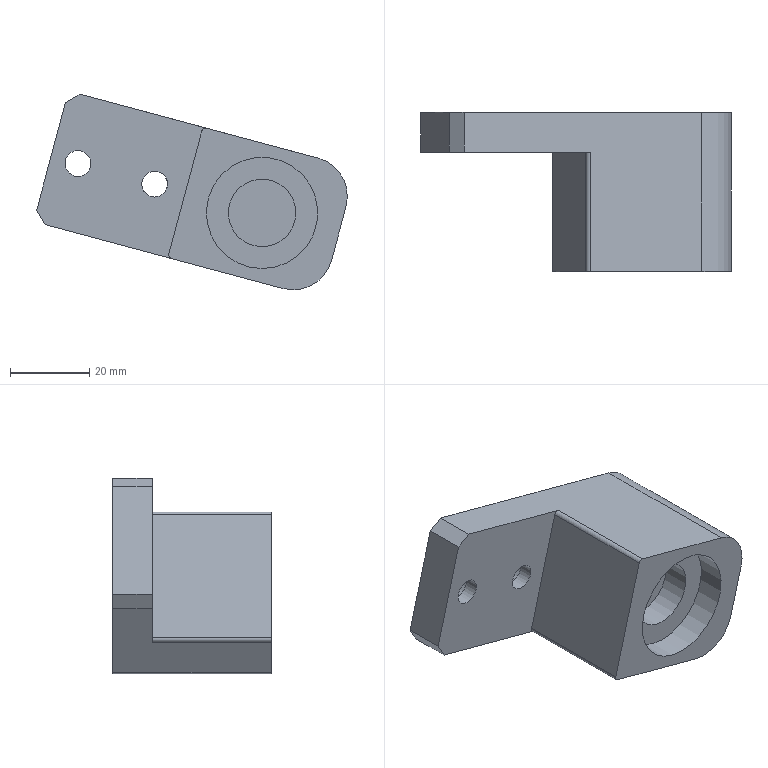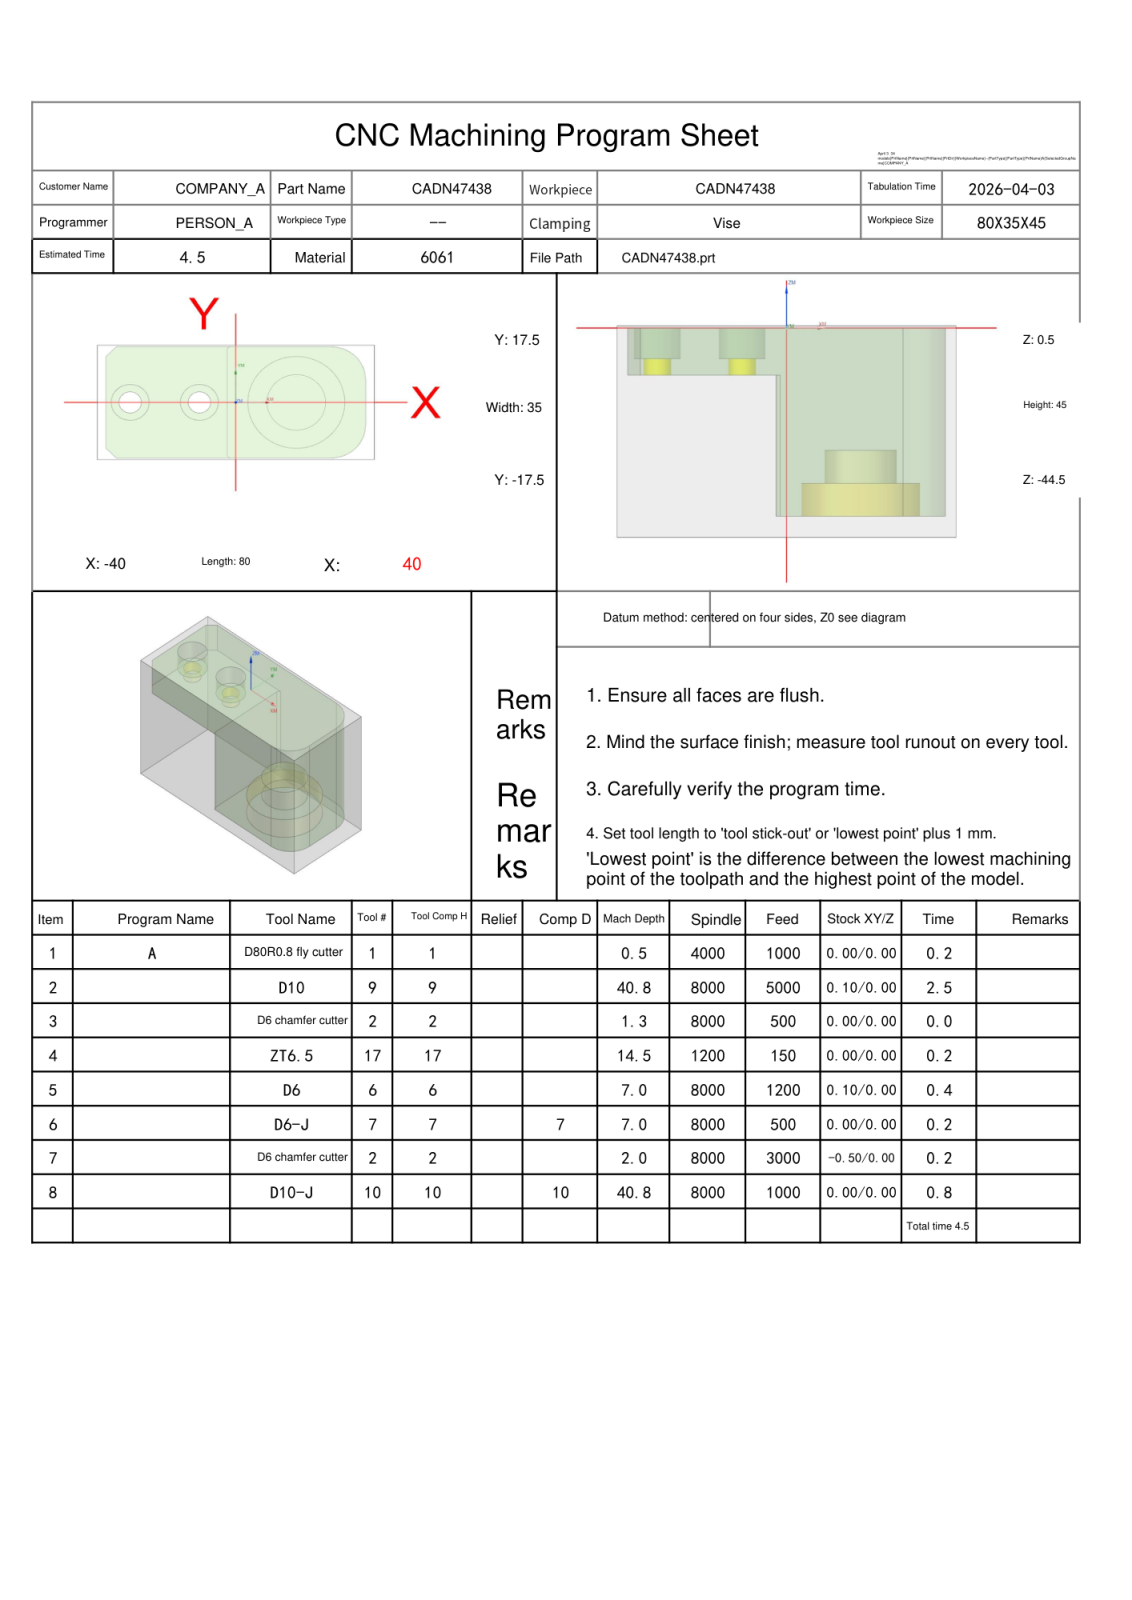NC program | NX | posted by the shop | part box 78.22 x 40 x 49.229 mm
Whole program:
%
O0001
(Machine time: 6.06 MIN)
(===Total Tool:7===)
(T1=D80R0.8 fly cutter D=80.  R=0.8  D-  H01 Z=-0.   )
(T9=D10     D=10.  R=0.   D-  H09 Z=-40.3 )
(T2=D6 chamfer cutter   D=6.   R=0.   D-  H02 Z=-1.5  )
(T17=ZT6.5  D=6.5  DR_a=118 D-  H17 Z=-13.95)
(T6=D6      D=6.   R=0.   D-  H06 Z=-6.5  )
(T7=D6-J    D=6.   R=0.   D7  H07 Z=-6.5  )
(T10=D10-J  D=10.  R=0.   D10 H10 Z=-40.3 )
G80 G90 G17 G49 G40
G91 G28 Z0
M01
N1 T01 M06
(D80R0.8 fly cutter  D=80. R=0.8 H=01 ce=0.00 di=0.00)
G00 G90 G54 X82.5 Y0.0 M03 S4000
G43 H01 Z20.
M08
Z2.
G01 Z0.0 F1000.
X77.5
X-77.5
X-82.5
Z2.
G00 Z20.
G91 G28 Z0.0
M05
M09
G91 G28 Z0.0
M01
N2 T09 M06
(D10  D=10. R=0. H=09 ce=0.10 di=0.00)
G00 G90 G54 X-3.5 Y-22.1 M03 S8000
G43 H09 Z20.
M08
Z.5
G01 X-34.5 Z.398 F5000.
G02 X-38.106 Y-20.606 Z.385 I0.0 J5.1
G01 X-41.106 Y-17.606 Z.371
G02 X-42.6 Y-14. Z.357 I3.606 J3.606
G01 Y14. Z.265
G02 X-41.106 Y17.606 Z.252 I5.1 J0.0
G01 X-38.106 Y20.606 Z.238
G02 X-34.5 Y22.1 Z.225 I3.606 J-3.606
G01 X27.5 Z.02
G02 X42.6 Y7. Z-.058 I0.0 J-15.1
G01 Y-7. Z-.104
G02 X27.5 Y-22.1 Z-.182 I-15.1 J0.0
G01 X-34.5 Z-.387
G02 X-38.106 Y-20.606 Z-.4 I0.0 J5.1
G01 X-41.106 Y-17.606 Z-.414
G02 X-42.6 Y-14. Z-.427 I3.606 J3.606
G01 Y14. Z-.52
G02 X-41.106 Y17.606 Z-.533 I5.1 J0.0
G01 X-38.106 Y20.606 Z-.547
G02 X-34.5 Y22.1 Z-.56 I3.606 J-3.606
G01 X27.5 Z-.764
G02 X42.6 Y7. Z-.843 I0.0 J-15.1
G01 Y-7. Z-.889
G02 X27.5 Y-22.1 Z-.967 I-15.1 J0.0
G01 X-34.5 Z-1.171
G02 X-38.106 Y-20.606 Z-1.185 I0.0 J5.1
G01 X-41.106 Y-17.606 Z-1.199
G02 X-42.6 Y-14. Z-1.212 I3.606 J3.606
G01 Y14. Z-1.304
G02 X-41.106 Y17.606 Z-1.317 I5.1 J0.0
G01 X-38.106 Y20.606 Z-1.331
G02 X-34.5 Y22.1 Z-1.345 I3.606 J-3.606
G01 X27.5 Z-1.549
G02 X42.6 Y7. Z-1.627 I0.0 J-15.1
G01 Y-7. Z-1.673
G02 X27.5 Y-22.1 Z-1.752 I-15.1 J0.0
G01 X-34.5 Z-1.956
G02 X-38.106 Y-20.606 Z-1.969 I0.0 J5.1
G01 X-41.106 Y-17.606 Z-1.983
G02 X-42.6 Y-14. Z-1.996 I3.606 J3.606
G01 Y14. Z-2.089
G02 X-41.106 Y17.606 Z-2.102 I5.1 J0.0
G01 X-38.106 Y20.606 Z-2.116
G02 X-34.5 Y22.1 Z-2.129 I3.606 J-3.606
G01 X27.5 Z-2.334
G02 X42.6 Y7. Z-2.412 I0.0 J-15.1
G01 Y-7. Z-2.458
G02 X27.5 Y-22.1 Z-2.536 I-15.1 J0.0
G01 X-34.5 Z-2.741
G02 X-38.106 Y-20.606 Z-2.754 I0.0 J5.1
G01 X-41.106 Y-17.606 Z-2.768
G02 X-42.6 Y-14. Z-2.781 I3.606 J3.606
G01 Y14. Z-2.873
G02 X-41.106 Y17.606 Z-2.887 I5.1 J0.0
G01 X-38.106 Y20.606 Z-2.901
G02 X-34.5 Y22.1 Z-2.914 I3.606 J-3.606
G01 X27.5 Z-3.118
G02 X42.6 Y7. Z-3.196 I0.0 J-15.1
G01 Y-7. Z-3.243
G02 X27.5 Y-22.1 Z-3.321 I-15.1 J0.0
G01 X-34.5 Z-3.525
G02 X-38.106 Y-20.606 Z-3.539 I0.0 J5.1
G01 X-41.106 Y-17.606 Z-3.552
G02 X-42.6 Y-14. Z-3.566 I3.606 J3.606
G01 Y14. Z-3.658
G02 X-41.106 Y17.606 Z-3.671 I5.1 J0.0
G01 X-38.106 Y20.606 Z-3.685
G02 X-34.5 Y22.1 Z-3.698 I3.606 J-3.606
G01 X27.5 Z-3.903
G02 X42.6 Y7. Z-3.981 I0.0 J-15.1
G01 Y-7. Z-4.027
G02 X27.5 Y-22.1 Z-4.105 I-15.1 J0.0
G01 X-34.5 Z-4.31
G02 X-38.106 Y-20.606 Z-4.323 I0.0 J5.1
G01 X-41.106 Y-17.606 Z-4.337
G02 X-42.6 Y-14. Z-4.35 I3.606 J3.606
G01 Y14. Z-4.443
G02 X-41.106 Y17.606 Z-4.456 I5.1 J0.0
G01 X-38.106 Y20.606 Z-4.47
G02 X-34.5 Y22.1 Z-4.483 I3.606 J-3.606
G01 X27.5 Z-4.687
G02 X42.6 Y7. Z-4.766 I0.0 J-15.1
G01 Y-7. Z-4.812
G02 X27.5 Y-22.1 Z-4.89 I-15.1 J0.0
G01 X-34.5 Z-5.095
G02 X-38.106 Y-20.606 Z-5.108 I0.0 J5.1
G01 X-41.106 Y-17.606 Z-5.122
G02 X-42.6 Y-14. Z-5.135 I3.606 J3.606
G01 Y14. Z-5.227
G02 X-41.106 Y17.606 Z-5.24 I5.1 J0.0
G01 X-38.106 Y20.606 Z-5.254
G02 X-34.5 Y22.1 Z-5.268 I3.606 J-3.606
G01 X27.5 Z-5.472
G02 X42.6 Y7. Z-5.55 I0.0 J-15.1
G01 Y-7. Z-5.596
G02 X27.5 Y-22.1 Z-5.675 I-15.1 J0.0
G01 X-34.5 Z-5.879
G02 X-38.106 Y-20.606 Z-5.892 I0.0 J5.1
G01 X-41.106 Y-17.606 Z-5.906
G02 X-42.6 Y-14. Z-5.92 I3.606 J3.606
G01 Y14. Z-6.012
G02 X-41.106 Y17.606 Z-6.025 I5.1 J0.0
G01 X-38.106 Y20.606 Z-6.039
G02 X-34.5 Y22.1 Z-6.052 I3.606 J-3.606
G01 X27.5 Z-6.257
G02 X42.6 Y7. Z-6.335 I0.0 J-15.1
G01 Y-7. Z-6.381
G02 X27.5 Y-22.1 Z-6.459 I-15.1 J0.0
G01 X-34.5 Z-6.664
G02 X-38.106 Y-20.606 Z-6.677 I0.0 J5.1
G01 X-41.106 Y-17.606 Z-6.691
G02 X-42.6 Y-14. Z-6.704 I3.606 J3.606
G01 Y14. Z-6.796
G02 X-41.106 Y17.606 Z-6.81 I5.1 J0.0
G01 X-38.106 Y20.606 Z-6.824
G02 X-34.5 Y22.1 Z-6.837 I3.606 J-3.606
G01 X27.5 Z-7.041
G02 X42.6 Y7. Z-7.12 I0.0 J-15.1
G01 Y-7. Z-7.166
G02 X27.5 Y-22.1 Z-7.244 I-15.1 J0.0
G01 X-34.5 Z-7.448
G02 X-38.106 Y-20.606 Z-7.462 I0.0 J5.1
G01 X-41.106 Y-17.606 Z-7.476
G02 X-42.6 Y-14. Z-7.489 I3.606 J3.606
G01 Y14. Z-7.581
G02 X-41.106 Y17.606 Z-7.594 I5.1 J0.0
G01 X-38.106 Y20.606 Z-7.608
G02 X-34.5 Y22.1 Z-7.622 I3.606 J-3.606
G01 X27.5 Z-7.826
G02 X42.6 Y7. Z-7.904 I0.0 J-15.1
G01 Y-7. Z-7.95
G02 X27.5 Y-22.1 Z-8.029 I-15.1 J0.0
G01 X-34.5 Z-8.233
G02 X-38.106 Y-20.606 Z-8.246 I0.0 J5.1
G01 X-41.106 Y-17.606 Z-8.26
G02 X-42.6 Y-14. Z-8.273 I3.606 J3.606
G01 Y14. Z-8.366
G02 X-41.106 Y17.606 Z-8.379 I5.1 J0.0
G01 X-38.106 Y20.606 Z-8.393
G02 X-34.5 Y22.1 Z-8.406 I3.606 J-3.606
G01 X27.5 Z-8.611
G02 X42.6 Y7. Z-8.689 I0.0 J-15.1
G01 Y-7. Z-8.735
G02 X27.5 Y-22.1 Z-8.813 I-15.1 J0.0
G01 X-34.5 Z-9.018
G02 X-38.106 Y-20.606 Z-9.031 I0.0 J5.1
G01 X-41.106 Y-17.606 Z-9.045
G02 X-42.6 Y-14. Z-9.058 I3.606 J3.606
G01 Y14. Z-9.15
G02 X-41.106 Y17.606 Z-9.164 I5.1 J0.0
G01 X-38.106 Y20.606 Z-9.178
G02 X-34.5 Y22.1 Z-9.191 I3.606 J-3.606
G01 X27.5 Z-9.395
G02 X42.6 Y7. Z-9.473 I0.0 J-15.1
G01 Y-7. Z-9.52
G02 X27.5 Y-22.1 Z-9.598 I-15.1 J0.0
G01 X-34.5 Z-9.802
G02 X-38.106 Y-20.606 Z-9.815 I0.0 J5.1
G01 X-41.106 Y-17.606 Z-9.829
G02 X-42.6 Y-14. Z-9.843 I3.606 J3.606
G01 Y14. Z-9.935
G02 X-41.106 Y17.606 Z-9.948 I5.1 J0.0
G01 X-38.106 Y20.606 Z-9.962
G02 X-34.5 Y22.1 Z-9.975 I3.606 J-3.606
G01 X27.5 Z-10.18
G02 X42.6 Y7. Z-10.258 I0.0 J-15.1
G01 Y-7. Z-10.304
G02 X27.5 Y-22.1 Z-10.382 I-15.1 J0.0
G01 X-34.5 Z-10.587
G02 X-38.106 Y-20.606 Z-10.6 I0.0 J5.1
G01 X-41.106 Y-17.606 Z-10.614
G02 X-42.6 Y-14. Z-10.627 I3.606 J3.606
G01 Y14. Z-10.72
G02 X-41.106 Y17.606 Z-10.733 I5.1 J0.0
G01 X-38.106 Y20.606 Z-10.747
G02 X-34.5 Y22.1 Z-10.76 I3.606 J-3.606
G01 X27.5 Z-10.964
G02 X42.6 Y7. Z-11.043 I0.0 J-15.1
G01 Y-7. Z-11.089
G02 X27.5 Y-22.1 Z-11.167 I-15.1 J0.0
G01 X-34.5 Z-11.371
G02 X-38.106 Y-20.606 Z-11.385 I0.0 J5.1
G01 X-41.106 Y-17.606 Z-11.399
G02 X-42.6 Y-14. Z-11.412 I3.606 J3.606
G01 Y14. Z-11.504
G02 X-41.106 Y17.606 Z-11.517 I5.1 J0.0
G01 X-38.106 Y20.606 Z-11.531
G02 X-34.5 Y22.1 Z-11.545 I3.606 J-3.606
G01 X27.5 Z-11.749
G02 X42.6 Y7. Z-11.827 I0.0 J-15.1
G01 Y-7. Z-11.873
G02 X27.5 Y-22.1 Z-11.952 I-15.1 J0.0
G01 X-34.5 Z-12.156
G02 X-38.106 Y-20.606 Z-12.169 I0.0 J5.1
G01 X-41.106 Y-17.606 Z-12.183
G02 X-42.6 Y-14. Z-12.196 I3.606 J3.606
G01 Y14. Z-12.289
G02 X-41.106 Y17.606 Z-12.302 I5.1 J0.0
G01 X-38.106 Y20.606 Z-12.316
G02 X-34.5 Y22.1 Z-12.329 I3.606 J-3.606
G01 X27.5 Z-12.534
G02 X42.6 Y7. Z-12.612 I0.0 J-15.1
G01 Y-7. Z-12.658
G02 X27.5 Y-22.1 Z-12.736 I-15.1 J0.0
G01 X-34.5 Z-12.941
G02 X-38.106 Y-20.606 Z-12.954 I0.0 J5.1
G01 X-41.106 Y-17.606 Z-12.968
G02 X-42.6 Y-14. Z-12.981 I3.606 J3.606
G01 Y14. Z-13.073
G02 X-41.106 Y17.606 Z-13.087 I5.1 J0.0
G01 X-38.106 Y20.606 Z-13.101
G02 X-34.5 Y22.1 Z-13.114 I3.606 J-3.606
G01 X27.5 Z-13.318
G02 X42.6 Y7. Z-13.396 I0.0 J-15.1
G01 Y-7. Z-13.443
G02 X27.5 Y-22.1 Z-13.521 I-15.1 J0.0
G01 X-34.5 Z-13.725
G02 X-38.106 Y-20.606 Z-13.739 I0.0 J5.1
G01 X-41.106 Y-17.606 Z-13.752
G02 X-42.6 Y-14. Z-13.766 I3.606 J3.606
G01 Y14. Z-13.858
G02 X-41.106 Y17.606 Z-13.871 I5.1 J0.0
G01 X-38.106 Y20.606 Z-13.885
G02 X-34.5 Y22.1 Z-13.898 I3.606 J-3.606
G01 X27.5 Z-14.103
G02 X42.6 Y7. Z-14.181 I0.0 J-15.1
G01 Y-7. Z-14.227
G02 X27.5 Y-22.1 Z-14.305 I-15.1 J0.0
G01 X-34.5 Z-14.51
G02 X-38.106 Y-20.606 Z-14.523 I0.0 J5.1
G01 X-41.106 Y-17.606 Z-14.537
G02 X-42.6 Y-14. Z-14.55 I3.606 J3.606
G01 Y14. Z-14.643
G02 X-41.106 Y17.606 Z-14.656 I5.1 J0.0
G01 X-38.106 Y20.606 Z-14.67
G02 X-34.5 Y22.1 Z-14.683 I3.606 J-3.606
G01 X27.5 Z-14.887
G02 X42.6 Y7. Z-14.966 I0.0 J-15.1
G01 Y-7. Z-15.012
G02 X27.5 Y-22.1 Z-15.09 I-15.1 J0.0
G01 X-34.5 Z-15.295
G02 X-38.106 Y-20.606 Z-15.308 I0.0 J5.1
G01 X-41.106 Y-17.606 Z-15.322
G02 X-42.6 Y-14. Z-15.335 I3.606 J3.606
G01 Y14. Z-15.427
G02 X-41.106 Y17.606 Z-15.44 I5.1 J0.0
G01 X-38.106 Y20.606 Z-15.454
G02 X-34.5 Y22.1 Z-15.468 I3.606 J-3.606
G01 X27.5 Z-15.672
G02 X42.6 Y7. Z-15.75 I0.0 J-15.1
G01 Y-7. Z-15.796
G02 X27.5 Y-22.1 Z-15.875 I-15.1 J0.0
G01 X-34.5 Z-16.079
G02 X-38.106 Y-20.606 Z-16.092 I0.0 J5.1
G01 X-41.106 Y-17.606 Z-16.106
G02 X-42.6 Y-14. Z-16.12 I3.606 J3.606
G01 Y14. Z-16.212
G02 X-41.106 Y17.606 Z-16.225 I5.1 J0.0
G01 X-38.106 Y20.606 Z-16.239
G02 X-34.5 Y22.1 Z-16.252 I3.606 J-3.606
G01 X27.5 Z-16.457
G02 X42.6 Y7. Z-16.535 I0.0 J-15.1
G01 Y-7. Z-16.581
G02 X27.5 Y-22.1 Z-16.659 I-15.1 J0.0
G01 X-34.5 Z-16.864
G02 X-38.106 Y-20.606 Z-16.877 I0.0 J5.1
G01 X-41.106 Y-17.606 Z-16.891
G02 X-42.6 Y-14. Z-16.904 I3.606 J3.606
G01 Y14. Z-16.996
G02 X-41.106 Y17.606 Z-17.01 I5.1 J0.0
G01 X-38.106 Y20.606 Z-17.024
G02 X-34.5 Y22.1 Z-17.037 I3.606 J-3.606
G01 X27.5 Z-17.241
G02 X42.6 Y7. Z-17.32 I0.0 J-15.1
G01 Y-7. Z-17.366
G02 X27.5 Y-22.1 Z-17.444 I-15.1 J0.0
G01 X-34.5 Z-17.648
G02 X-38.106 Y-20.606 Z-17.662 I0.0 J5.1
G01 X-41.106 Y-17.606 Z-17.676
G02 X-42.6 Y-14. Z-17.689 I3.606 J3.606
G01 Y14. Z-17.781
G02 X-41.106 Y17.606 Z-17.794 I5.1 J0.0
G01 X-38.106 Y20.606 Z-17.808
G02 X-34.5 Y22.1 Z-17.822 I3.606 J-3.606
G01 X27.5 Z-18.026
G02 X42.6 Y7. Z-18.104 I0.0 J-15.1
G01 Y-7. Z-18.15
G02 X27.5 Y-22.1 Z-18.229 I-15.1 J0.0
G01 X-34.5 Z-18.433
G02 X-38.106 Y-20.606 Z-18.446 I0.0 J5.1
G01 X-41.106 Y-17.606 Z-18.46
G02 X-42.6 Y-14. Z-18.473 I3.606 J3.606
G01 Y14. Z-18.566
G02 X-41.106 Y17.606 Z-18.579 I5.1 J0.0
G01 X-38.106 Y20.606 Z-18.593
G02 X-34.5 Y22.1 Z-18.606 I3.606 J-3.606
G01 X27.5 Z-18.811
G02 X42.6 Y7. Z-18.889 I0.0 J-15.1
G01 Y-7. Z-18.935
G02 X27.5 Y-22.1 Z-19.013 I-15.1 J0.0
G01 X-34.5 Z-19.218
G02 X-38.106 Y-20.606 Z-19.231 I0.0 J5.1
G01 X-41.106 Y-17.606 Z-19.245
G02 X-42.6 Y-14. Z-19.258 I3.606 J3.606
G01 Y14. Z-19.35
G02 X-41.106 Y17.606 Z-19.364 I5.1 J0.0
G01 X-38.106 Y20.606 Z-19.378
G02 X-34.5 Y22.1 Z-19.391 I3.606 J-3.606
G01 X27.5 Z-19.595
G02 X42.6 Y7. Z-19.673 I0.0 J-15.1
G01 Y-7. Z-19.72
G02 X27.5 Y-22.1 Z-19.798 I-15.1 J0.0
G01 X-34.5 Z-20.002
G02 X-38.106 Y-20.606 Z-20.015 I0.0 J5.1
G01 X-41.106 Y-17.606 Z-20.029
G02 X-42.6 Y-14. Z-20.043 I3.606 J3.606
G01 Y14. Z-20.135
G02 X-41.106 Y17.606 Z-20.148 I5.1 J0.0
G01 X-38.106 Y20.606 Z-20.162
G02 X-34.5 Y22.1 Z-20.175 I3.606 J-3.606
G01 X27.5 Z-20.38
G02 X42.6 Y7. Z-20.458 I0.0 J-15.1
G01 Y-7. Z-20.504
G02 X27.5 Y-22.1 Z-20.582 I-15.1 J0.0
G01 X-34.5 Z-20.787
G02 X-38.106 Y-20.606 Z-20.8 I0.0 J5.1
G01 X-41.106 Y-17.606 Z-20.814
G02 X-42.6 Y-14. Z-20.827 I3.606 J3.606
G01 Y14. Z-20.92
G02 X-41.106 Y17.606 Z-20.933 I5.1 J0.0
G01 X-38.106 Y20.606 Z-20.947
G02 X-34.5 Y22.1 Z-20.96 I3.606 J-3.606
G01 X27.5 Z-21.164
G02 X42.6 Y7. Z-21.243 I0.0 J-15.1
G01 Y-7. Z-21.289
G02 X27.5 Y-22.1 Z-21.367 I-15.1 J0.0
G01 X-34.5 Z-21.571
G02 X-38.106 Y-20.606 Z-21.585 I0.0 J5.1
G01 X-41.106 Y-17.606 Z-21.599
G02 X-42.6 Y-14. Z-21.612 I3.606 J3.606
G01 Y14. Z-21.704
G02 X-41.106 Y17.606 Z-21.717 I5.1 J0.0
G01 X-38.106 Y20.606 Z-21.731
G02 X-34.5 Y22.1 Z-21.745 I3.606 J-3.606
G01 X27.5 Z-21.949
G02 X42.6 Y7. Z-22.027 I0.0 J-15.1
G01 Y-7. Z-22.073
G02 X27.5 Y-22.1 Z-22.152 I-15.1 J0.0
G01 X-34.5 Z-22.356
G02 X-38.106 Y-20.606 Z-22.369 I0.0 J5.1
G01 X-41.106 Y-17.606 Z-22.383
G02 X-42.6 Y-14. Z-22.396 I3.606 J3.606
G01 Y14. Z-22.489
G02 X-41.106 Y17.606 Z-22.502 I5.1 J0.0
G01 X-38.106 Y20.606 Z-22.516
G02 X-34.5 Y22.1 Z-22.529 I3.606 J-3.606
G01 X27.5 Z-22.734
G02 X42.6 Y7. Z-22.812 I0.0 J-15.1
G01 Y-7. Z-22.858
G02 X27.5 Y-22.1 Z-22.936 I-15.1 J0.0
G01 X-34.5 Z-23.141
G02 X-38.106 Y-20.606 Z-23.154 I0.0 J5.1
G01 X-41.106 Y-17.606 Z-23.168
G02 X-42.6 Y-14. Z-23.181 I3.606 J3.606
G01 Y14. Z-23.273
G02 X-41.106 Y17.606 Z-23.287 I5.1 J0.0
G01 X-38.106 Y20.606 Z-23.301
G02 X-34.5 Y22.1 Z-23.314 I3.606 J-3.606
G01 X27.5 Z-23.518
G02 X42.6 Y7. Z-23.596 I0.0 J-15.1
G01 Y-7. Z-23.643
G02 X27.5 Y-22.1 Z-23.721 I-15.1 J0.0
G01 X-34.5 Z-23.925
G02 X-38.106 Y-20.606 Z-23.939 I0.0 J5.1
G01 X-41.106 Y-17.606 Z-23.952
G02 X-42.6 Y-14. Z-23.966 I3.606 J3.606
G01 Y14. Z-24.058
G02 X-41.106 Y17.606 Z-24.071 I5.1 J0.0
G01 X-38.106 Y20.606 Z-24.085
G02 X-34.5 Y22.1 Z-24.098 I3.606 J-3.606
G01 X27.5 Z-24.303
G02 X42.6 Y7. Z-24.381 I0.0 J-15.1
G01 Y-7. Z-24.427
G02 X27.5 Y-22.1 Z-24.505 I-15.1 J0.0
G01 X-34.5 Z-24.71
G02 X-38.106 Y-20.606 Z-24.723 I0.0 J5.1
G01 X-41.106 Y-17.606 Z-24.737
G02 X-42.6 Y-14. Z-24.75 I3.606 J3.606
G01 Y14. Z-24.843
G02 X-41.106 Y17.606 Z-24.856 I5.1 J0.0
G01 X-38.106 Y20.606 Z-24.87
G02 X-34.5 Y22.1 Z-24.883 I3.606 J-3.606
G01 X27.5 Z-25.087
G02 X42.6 Y7. Z-25.166 I0.0 J-15.1
G01 Y-7. Z-25.212
G02 X27.5 Y-22.1 Z-25.29 I-15.1 J0.0
G01 X-34.5 Z-25.495
G02 X-38.106 Y-20.606 Z-25.508 I0.0 J5.1
G01 X-41.106 Y-17.606 Z-25.522
G02 X-42.6 Y-14. Z-25.535 I3.606 J3.606
G01 Y14. Z-25.627
G02 X-41.106 Y17.606 Z-25.64 I5.1 J0.0
G01 X-38.106 Y20.606 Z-25.654
G02 X-34.5 Y22.1 Z-25.668 I3.606 J-3.606
G01 X27.5 Z-25.872
G02 X42.6 Y7. Z-25.95 I0.0 J-15.1
G01 Y-7. Z-25.996
G02 X27.5 Y-22.1 Z-26.075 I-15.1 J0.0
G01 X-34.5 Z-26.279
G02 X-38.106 Y-20.606 Z-26.292 I0.0 J5.1
G01 X-41.106 Y-17.606 Z-26.306
G02 X-42.6 Y-14. Z-26.32 I3.606 J3.606
G01 Y14. Z-26.412
G02 X-41.106 Y17.606 Z-26.425 I5.1 J0.0
G01 X-38.106 Y20.606 Z-26.439
G02 X-34.5 Y22.1 Z-26.452 I3.606 J-3.606
G01 X27.5 Z-26.657
G02 X42.6 Y7. Z-26.735 I0.0 J-15.1
G01 Y-7. Z-26.781
G02 X27.5 Y-22.1 Z-26.859 I-15.1 J0.0
G01 X-34.5 Z-27.064
G02 X-38.106 Y-20.606 Z-27.077 I0.0 J5.1
G01 X-41.106 Y-17.606 Z-27.091
G02 X-42.6 Y-14. Z-27.104 I3.606 J3.606
G01 Y14. Z-27.196
G02 X-41.106 Y17.606 Z-27.21 I5.1 J0.0
G01 X-38.106 Y20.606 Z-27.224
G02 X-34.5 Y22.1 Z-27.237 I3.606 J-3.606
G01 X27.5 Z-27.441
G02 X42.6 Y7. Z-27.52 I0.0 J-15.1
G01 Y-7. Z-27.566
G02 X27.5 Y-22.1 Z-27.644 I-15.1 J0.0
G01 X-34.5 Z-27.848
G02 X-38.106 Y-20.606 Z-27.862 I0.0 J5.1
G01 X-41.106 Y-17.606 Z-27.876
G02 X-42.6 Y-14. Z-27.889 I3.606 J3.606
G01 Y14. Z-27.981
G02 X-41.106 Y17.606 Z-27.994 I5.1 J0.0
G01 X-38.106 Y20.606 Z-28.008
G02 X-34.5 Y22.1 Z-28.022 I3.606 J-3.606
G01 X27.5 Z-28.226
G02 X42.6 Y7. Z-28.304 I0.0 J-15.1
G01 Y-7. Z-28.35
G02 X27.5 Y-22.1 Z-28.429 I-15.1 J0.0
G01 X-34.5 Z-28.633
G02 X-38.106 Y-20.606 Z-28.646 I0.0 J5.1
G01 X-41.106 Y-17.606 Z-28.66
G02 X-42.6 Y-14. Z-28.673 I3.606 J3.606
G01 Y14. Z-28.766
G02 X-41.106 Y17.606 Z-28.779 I5.1 J0.0
G01 X-38.106 Y20.606 Z-28.793
G02 X-34.5 Y22.1 Z-28.806 I3.606 J-3.606
G01 X27.5 Z-29.011
G02 X42.6 Y7. Z-29.089 I0.0 J-15.1
G01 Y-7. Z-29.135
G02 X27.5 Y-22.1 Z-29.213 I-15.1 J0.0
G01 X-34.5 Z-29.418
G02 X-38.106 Y-20.606 Z-29.431 I0.0 J5.1
G01 X-41.106 Y-17.606 Z-29.445
G02 X-42.6 Y-14. Z-29.458 I3.606 J3.606
G01 Y14. Z-29.55
G02 X-41.106 Y17.606 Z-29.564 I5.1 J0.0
G01 X-38.106 Y20.606 Z-29.578
G02 X-34.5 Y22.1 Z-29.591 I3.606 J-3.606
G01 X27.5 Z-29.795
G02 X42.6 Y7. Z-29.873 I0.0 J-15.1
G01 Y-7. Z-29.92
G02 X27.5 Y-22.1 Z-29.998 I-15.1 J0.0
G01 X-34.5 Z-30.202
G02 X-38.106 Y-20.606 Z-30.215 I0.0 J5.1
G01 X-41.106 Y-17.606 Z-30.229
G02 X-42.6 Y-14. Z-30.243 I3.606 J3.606
G01 Y14. Z-30.335
G02 X-41.106 Y17.606 Z-30.348 I5.1 J0.0
G01 X-38.106 Y20.606 Z-30.362
G02 X-34.5 Y22.1 Z-30.375 I3.606 J-3.606
G01 X27.5 Z-30.58
G02 X42.6 Y7. Z-30.658 I0.0 J-15.1
G01 Y-7. Z-30.704
G02 X27.5 Y-22.1 Z-30.782 I-15.1 J0.0
G01 X-34.5 Z-30.987
G02 X-38.106 Y-20.606 Z-31. I0.0 J5.1
G01 X-41.106 Y-17.606 Z-31.014
G02 X-42.6 Y-14. Z-31.027 I3.606 J3.606
G01 Y14. Z-31.12
G02 X-41.106 Y17.606 Z-31.133 I5.1 J0.0
G01 X-38.106 Y20.606 Z-31.147
G02 X-34.5 Y22.1 Z-31.16 I3.606 J-3.606
G01 X27.5 Z-31.364
G02 X42.6 Y7. Z-31.443 I0.0 J-15.1
G01 Y-7. Z-31.489
G02 X27.5 Y-22.1 Z-31.567 I-15.1 J0.0
G01 X-34.5 Z-31.771
G02 X-38.106 Y-20.606 Z-31.785 I0.0 J5.1
G01 X-41.106 Y-17.606 Z-31.799
G02 X-42.6 Y-14. Z-31.812 I3.606 J3.606
G01 Y14. Z-31.904
G02 X-41.106 Y17.606 Z-31.917 I5.1 J0.0
G01 X-38.106 Y20.606 Z-31.931
G02 X-34.5 Y22.1 Z-31.945 I3.606 J-3.606
G01 X27.5 Z-32.149
G02 X42.6 Y7. Z-32.227 I0.0 J-15.1
G01 Y-7. Z-32.273
G02 X27.5 Y-22.1 Z-32.352 I-15.1 J0.0
G01 X-34.5 Z-32.556
G02 X-38.106 Y-20.606 Z-32.569 I0.0 J5.1
G01 X-41.106 Y-17.606 Z-32.583
G02 X-42.6 Y-14. Z-32.596 I3.606 J3.606
G01 Y14. Z-32.689
G02 X-41.106 Y17.606 Z-32.702 I5.1 J0.0
G01 X-38.106 Y20.606 Z-32.716
G02 X-34.5 Y22.1 Z-32.729 I3.606 J-3.606
G01 X27.5 Z-32.934
G02 X42.6 Y7. Z-33.012 I0.0 J-15.1
G01 Y-7. Z-33.058
G02 X27.5 Y-22.1 Z-33.136 I-15.1 J0.0
G01 X-34.5 Z-33.341
G02 X-38.106 Y-20.606 Z-33.354 I0.0 J5.1
G01 X-41.106 Y-17.606 Z-33.368
G02 X-42.6 Y-14. Z-33.381 I3.606 J3.606
G01 Y14. Z-33.473
G02 X-41.106 Y17.606 Z-33.487 I5.1 J0.0
G01 X-38.106 Y20.606 Z-33.501
G02 X-34.5 Y22.1 Z-33.514 I3.606 J-3.606
G01 X27.5 Z-33.718
G02 X42.6 Y7. Z-33.796 I0.0 J-15.1
G01 Y-7. Z-33.843
G02 X27.5 Y-22.1 Z-33.921 I-15.1 J0.0
G01 X-34.5 Z-34.125
G02 X-38.106 Y-20.606 Z-34.139 I0.0 J5.1
G01 X-41.106 Y-17.606 Z-34.152
G02 X-42.6 Y-14. Z-34.166 I3.606 J3.606
G01 Y14. Z-34.258
G02 X-41.106 Y17.606 Z-34.271 I5.1 J0.0
G01 X-38.106 Y20.606 Z-34.285
G02 X-34.5 Y22.1 Z-34.298 I3.606 J-3.606
G01 X27.5 Z-34.503
G02 X42.6 Y7. Z-34.581 I0.0 J-15.1
G01 Y-7. Z-34.627
G02 X27.5 Y-22.1 Z-34.705 I-15.1 J0.0
G01 X-34.5 Z-34.91
G02 X-38.106 Y-20.606 Z-34.923 I0.0 J5.1
G01 X-41.106 Y-17.606 Z-34.937
G02 X-42.6 Y-14. Z-34.95 I3.606 J3.606
G01 Y14. Z-35.043
G02 X-41.106 Y17.606 Z-35.056 I5.1 J0.0
G01 X-38.106 Y20.606 Z-35.07
G02 X-34.5 Y22.1 Z-35.083 I3.606 J-3.606
G01 X27.5 Z-35.287
G02 X42.6 Y7. Z-35.366 I0.0 J-15.1
G01 Y-7. Z-35.412
G02 X27.5 Y-22.1 Z-35.49 I-15.1 J0.0
G01 X-34.5 Z-35.695
G02 X-38.106 Y-20.606 Z-35.708 I0.0 J5.1
G01 X-41.106 Y-17.606 Z-35.722
G02 X-42.6 Y-14. Z-35.735 I3.606 J3.606
G01 Y14. Z-35.827
G02 X-41.106 Y17.606 Z-35.84 I5.1 J0.0
G01 X-38.106 Y20.606 Z-35.854
G02 X-34.5 Y22.1 Z-35.868 I3.606 J-3.606
G01 X27.5 Z-36.072
G02 X42.6 Y7. Z-36.15 I0.0 J-15.1
G01 Y-7. Z-36.196
G02 X27.5 Y-22.1 Z-36.275 I-15.1 J0.0
G01 X-34.5 Z-36.479
G02 X-38.106 Y-20.606 Z-36.492 I0.0 J5.1
G01 X-41.106 Y-17.606 Z-36.506
G02 X-42.6 Y-14. Z-36.52 I3.606 J3.606
G01 Y14. Z-36.612
G02 X-41.106 Y17.606 Z-36.625 I5.1 J0.0
G01 X-38.106 Y20.606 Z-36.639
G02 X-34.5 Y22.1 Z-36.652 I3.606 J-3.606
G01 X27.5 Z-36.857
G02 X42.6 Y7. Z-36.935 I0.0 J-15.1
G01 Y-7. Z-36.981
G02 X27.5 Y-22.1 Z-37.059 I-15.1 J0.0
G01 X-34.5 Z-37.264
G02 X-38.106 Y-20.606 Z-37.277 I0.0 J5.1
G01 X-41.106 Y-17.606 Z-37.291
G02 X-42.6 Y-14. Z-37.304 I3.606 J3.606
G01 Y14. Z-37.396
G02 X-41.106 Y17.606 Z-37.41 I5.1 J0.0
G01 X-38.106 Y20.606 Z-37.424
G02 X-34.5 Y22.1 Z-37.437 I3.606 J-3.606
G01 X27.5 Z-37.641
G02 X42.6 Y7. Z-37.72 I0.0 J-15.1
G01 Y-7. Z-37.766
G02 X27.5 Y-22.1 Z-37.844 I-15.1 J0.0
G01 X-34.5 Z-38.048
G02 X-38.106 Y-20.606 Z-38.062 I0.0 J5.1
G01 X-41.106 Y-17.606 Z-38.076
G02 X-42.6 Y-14. Z-38.089 I3.606 J3.606
G01 Y14. Z-38.181
G02 X-41.106 Y17.606 Z-38.194 I5.1 J0.0
G01 X-38.106 Y20.606 Z-38.208
G02 X-34.5 Y22.1 Z-38.222 I3.606 J-3.606
G01 X27.5 Z-38.426
G02 X42.6 Y7. Z-38.504 I0.0 J-15.1
G01 Y-7. Z-38.55
G02 X27.5 Y-22.1 Z-38.629 I-15.1 J0.0
G01 X-34.5 Z-38.833
G02 X-38.106 Y-20.606 Z-38.846 I0.0 J5.1
G01 X-41.106 Y-17.606 Z-38.86
G02 X-42.6 Y-14. Z-38.873 I3.606 J3.606
G01 Y14. Z-38.966
G02 X-41.106 Y17.606 Z-38.979 I5.1 J0.0
G01 X-38.106 Y20.606 Z-38.993
G02 X-34.5 Y22.1 Z-39.006 I3.606 J-3.606
G01 X27.5 Z-39.211
G02 X42.6 Y7. Z-39.289 I0.0 J-15.1
G01 Y-7. Z-39.335
G02 X27.5 Y-22.1 Z-39.413 I-15.1 J0.0
G01 X-34.5 Z-39.618
G02 X-38.106 Y-20.606 Z-39.631 I0.0 J5.1
G01 X-41.106 Y-17.606 Z-39.645
G02 X-42.6 Y-14. Z-39.658 I3.606 J3.606
G01 Y14. Z-39.75
G02 X-41.106 Y17.606 Z-39.764 I5.1 J0.0
G01 X-38.106 Y20.606 Z-39.778
G02 X-34.5 Y22.1 Z-39.791 I3.606 J-3.606
G01 X27.5 Z-39.995
G02 X42.6 Y7. Z-40.073 I0.0 J-15.1
G01 Y-7. Z-40.12
G02 X27.5 Y-22.1 Z-40.198 I-15.1 J0.0
G01 X-3.5 Z-40.3
X-34.5
G02 X-38.106 Y-20.606 I0.0 J5.1
G01 X-41.106 Y-17.606
G02 X-42.6 Y-14. I3.606 J3.606
G01 Y14.
G02 X-41.106 Y17.606 I5.1 J0.0
G01 X-38.106 Y20.606
G02 X-34.5 Y22.1 I3.606 J-3.606
G01 X27.5
G02 X42.6 Y7. I0.0 J-15.1
G01 Y-7.
G02 X27.5 Y-22.1 I-15.1 J0.0
G01 X-3.5
X-4.
Z-39.3
G00 Z20.
G91 G28 Z0.0
M05
M09
G91 G28 Z0.0
M01
N3 T02 M06
(D6 chamfer cutter  D=6. R=0. H=02 ce=0.00 di=0.00)
G00 G90 G54 X-10.5 Y0.0 M03 S8000
G43 H02 Z20.
M08
G98 G81 X-10.5 Y0.0 Z-.8 R1. F500.
X-30.5
G80
G00 Z20.
G91 G28 Z0.0
M05
M09
G91 G28 Z0.0
M01
N4 T17 M06
(ZT6.5 D=6.5 DR_a=118 H=17)
G00 G90 G54 X-10.5 Y0.0 M03 S1200
G43 H17 Z20.
M08
G98 G83 X-10.5 Y0.0 Z-13.953 R1. F150. Q2.
X-30.5
G80
G00 Z20.
G91 G28 Z0.0
M05
M09
G91 G28 Z0.0
M01
N5 T06 M06
(D6  D=6. R=0. H=06 ce=0.10 di=0.00)
G00 G90 G54 X-10.5 Y0.0 M03 S8000
G43 H06 Z20.
M08
Z.5
G03 X-10.541 Y-.311 I1.159 J-.311 F1200.
X-9.341 Y-1.511 I1.2 J0.0
X-8.182 Y-.621 I0.0 J1.2
X-8.182 Y-.621 Z0.0 I-2.318 J.621
X-8.182 Y-.621 Z-.5 I-2.318 J.621
X-8.182 Y-.621 Z-1. I-2.318 J.621
X-8.182 Y-.621 Z-1.5 I-2.318 J.621
X-8.182 Y-.621 Z-2. I-2.318 J.621
X-8.182 Y-.621 Z-2.5 I-2.318 J.621
X-8.182 Y-.621 Z-3. I-2.318 J.621
X-8.182 Y-.621 Z-3.5 I-2.318 J.621
X-8.182 Y-.621 Z-4. I-2.318 J.621
X-8.182 Y-.621 Z-4.5 I-2.318 J.621
X-8.182 Y-.621 Z-5. I-2.318 J.621
X-8.182 Y-.621 Z-5.5 I-2.318 J.621
X-8.182 Y-.621 Z-6. I-2.318 J.621
X-8.182 Y-.621 Z-6.5 I-2.318 J.621
X-8.1 Y0.0 I-2.318 J.621
X-10.5 Y2.4 I-2.4 J0.0
X-12.9 Y0.0 I0.0 J-2.4
X-10.5 Y-2.4 I2.4 J0.0
X-8.182 Y-.621 I0.0 J2.4
X-8.141 Y-.311 I-1.159 J.311
X-9.341 Y.889 I-1.2 J0.0
X-10.5 Y0.0 I0.0 J-1.2
G00 Z20.
X-30.5
Z.5
G03 X-30.541 Y-.311 I1.159 J-.311
X-29.341 Y-1.511 I1.2 J0.0
X-28.182 Y-.621 I0.0 J1.2
X-28.182 Y-.621 Z0.0 I-2.318 J.621
X-28.182 Y-.621 Z-.5 I-2.318 J.621
X-28.182 Y-.621 Z-1. I-2.318 J.621
X-28.182 Y-.621 Z-1.5 I-2.318 J.621
X-28.182 Y-.621 Z-2. I-2.318 J.621
X-28.182 Y-.621 Z-2.5 I-2.318 J.621
X-28.182 Y-.621 Z-3. I-2.318 J.621
X-28.182 Y-.621 Z-3.5 I-2.318 J.621
X-28.182 Y-.621 Z-4. I-2.318 J.621
X-28.182 Y-.621 Z-4.5 I-2.318 J.621
X-28.182 Y-.621 Z-5. I-2.318 J.621
X-28.182 Y-.621 Z-5.5 I-2.318 J.621
X-28.182 Y-.621 Z-6. I-2.318 J.621
X-28.182 Y-.621 Z-6.5 I-2.318 J.621
X-28.1 Y0.0 I-2.318 J.621
X-30.5 Y2.4 I-2.4 J0.0
X-32.9 Y0.0 I0.0 J-2.4
X-30.5 Y-2.4 I2.4 J0.0
X-28.182 Y-.621 I0.0 J2.4
X-28.141 Y-.311 I-1.159 J.311
X-29.341 Y.889 I-1.2 J0.0
X-30.5 Y0.0 I0.0 J-1.2
G00 Z20.
G91 G28 Z0.0
M05
M09
G91 G28 Z0.0
M01
N6 T07 M06
(D6-J  D=6. R=0. H=07 ce=0.00 di=0.00)
G00 G90 G54 X-10.5 Y0.0 M03 S8000
G43 H07 Z20.
M08
Z0.0
G41 D07
G01 X-10.52 Y-.199 F500.
X-10.527 Y-.326
G03 X-9.285 Y-1.568 I1.242 J0.0
X-8.085 Y-.647 I0.0 J1.242
X-8.085 Y-.647 Z-5. I-2.415 J.647
X-10.631 Y2.497 Z-6.5 I-2.415 J.647
X-13. Y0.0 I.131 J-2.497
X-10.5 Y-2.5 I2.5 J0.0
X-8. Y0.0 I0.0 J2.5
X-10.5 Y2.5 I-2.5 J0.0
G01 X-10.631 Y2.497
G03 X-11.808 Y1.256 I.065 J-1.24
X-10.699 Y.021 I1.242 J0.0
G01 G40 X-10.5 Y0.0
G00 Z20.
X-30.5
Z0.0
G41 D07
G01 X-30.52 Y-.199
X-30.527 Y-.326
G03 X-29.285 Y-1.568 I1.242 J0.0
X-28.085 Y-.647 I0.0 J1.242
X-28.085 Y-.647 Z-5. I-2.415 J.647
X-30.631 Y2.497 Z-6.5 I-2.415 J.647
X-33. Y0.0 I.131 J-2.497
X-30.5 Y-2.5 I2.5 J0.0
X-28. Y0.0 I0.0 J2.5
X-30.5 Y2.5 I-2.5 J0.0
G01 X-30.631 Y2.497
G03 X-31.808 Y1.256 I.065 J-1.24
X-30.699 Y.021 I1.242 J0.0
G01 G40 X-30.5 Y0.0
G00 Z20.
G91 G28 Z0.0
M05
M09
G91 G28 Z0.0
M01
N7 T02 M06
(D6 chamfer cutter  D=6. R=0. H=02 ce=0.00 di=0.00)
G00 G90 G54 X-3.75 Y18.828 M03 S8000
G43 H02 Z20.
M08
Z2.399
G01 Z-1.5 F3000.
G03 X-3.83 Y18.528 I.52 J-.3
X-3.53 Y18.008 I.6 J0.0
G01 X-3.5 Y18.
X27.5
G02 X38.5 Y7. I0.0 J-11.
G01 Y-7.
G02 X27.5 Y-18. I-11. J0.0
G01 X-34.5
X-34.759 Y-17.966
X-35. Y-17.866
X-35.207 Y-17.707
X-38.207 Y-14.707
X-38.366 Y-14.5
X-38.466 Y-14.259
X-38.5 Y-14.
Y14.
X-38.466 Y14.259
X-38.366 Y14.5
X-38.207 Y14.707
X-35.207 Y17.707
X-35. Y17.866
X-34.759 Y17.966
X-34.5 Y18.
X-3.5
X-3.47 Y18.008
G03 X-3.17 Y18.528 I-.3 J.52
X-3.25 Y18.828 I-.6 J0.0
G01 Z2.399
G00 Z20.
G00 G90 X-6.415 Y-2.878 M03 S8000
Z20.
Z2.5
G01 X-6.256 Y-2.649 Z2.398 F800.
X-6.02 Y-2.228 Z2.223
X-5.827 Y-1.786 Z2.047
X-5.676 Y-1.328 Z1.872
X-5.571 Y-.857 Z1.696
X-5.511 Y-.378 Z1.521
X-5.498 Y.104 Z1.345
X-5.531 Y.585 Z1.169
X-5.611 Y1.06 Z.994
X-5.736 Y1.526 Z.818
X-5.905 Y1.978 Z.643
X-6.116 Y2.411 Z.467
X-6.369 Y2.822 Z.292
X-6.66 Y3.207 Z.116
X-6.986 Y3.562 Z-.059
X-7.346 Y3.883 Z-.235
X-7.734 Y4.169 Z-.41
X-8.149 Y4.416 Z-.586
X-8.585 Y4.622 Z-.761
X-9.039 Y4.785 Z-.937
X-9.206 Y4.83 Z-1.
G03 X-10.5 Y5. I-1.294 J-4.83
X-15.5 Y0.0 I0.0 J-5.
X-10.5 Y-5. I5. J0.0
X-5.5 Y0.0 I0.0 J5.
X-9.206 Y4.83 I-5. J0.0
X-9.695 Y4.935 I-1.294 J-4.83
G01 Z1.5
G00 Z20.
X-26.415 Y-2.878
Z2.5
G01 X-26.256 Y-2.649 Z2.398
X-26.02 Y-2.228 Z2.223
X-25.827 Y-1.786 Z2.047
X-25.676 Y-1.328 Z1.872
X-25.571 Y-.857 Z1.696
X-25.511 Y-.378 Z1.521
X-25.498 Y.104 Z1.345
X-25.531 Y.585 Z1.169
X-25.611 Y1.06 Z.994
X-25.736 Y1.526 Z.818
X-25.905 Y1.978 Z.643
X-26.116 Y2.411 Z.467
X-26.369 Y2.822 Z.292
X-26.66 Y3.207 Z.116
X-26.986 Y3.562 Z-.059
X-27.346 Y3.883 Z-.235
X-27.734 Y4.169 Z-.41
X-28.149 Y4.416 Z-.586
X-28.585 Y4.622 Z-.761
X-29.039 Y4.785 Z-.937
X-29.206 Y4.83 Z-1.
G03 X-30.5 Y5. I-1.294 J-4.83
X-35.5 Y0.0 I0.0 J-5.
X-30.5 Y-5. I5. J0.0
X-25.5 Y0.0 I0.0 J5.
X-29.206 Y4.83 I-5. J0.0
X-29.695 Y4.935 I-1.294 J-4.83
G01 Z1.5
G00 Z20.
G91 G28 Z0.0
M05
M09
G91 G28 Z0.0
M01
N8 T10 M06
(D10-J  D=10. R=0. H=10 ce=0.00 di=0.00)
G00 G90 G54 X28.506 Y-23.169 M03 S8000
G43 H10 Z20.
M08
Z-12.933
G01 Z-13.433 F1000.
G41 D10
X28.5 Y-22.969
G03 X27.5 Y-22. I-1. J-.031
G01 X-34.5
G02 X-38.036 Y-20.536 I0.0 J5.
G01 X-41.036 Y-17.536
G02 X-42.5 Y-14. I3.536 J3.536
G01 Y14.
G02 X-41.036 Y17.536 I5. J0.0
G01 X-38.036 Y20.536
G02 X-34.5 Y22. I3.536 J-3.536
G01 X-1.5
X27.5
G02 X42.5 Y7. I0.0 J-15.
G01 Y-7.
G02 X27.5 Y-22. I-15. J0.0
G01 X27.
G03 X26. Y-23. I0.0 J-1.
G01 G40 Y-23.2
Z-12.933
G00 Z20.
X28.506 Y-23.169
Z-26.367
G01 Z-26.867
G41 D10
X28.5 Y-22.969
G03 X27.5 Y-22. I-1. J-.031
G01 X-34.5
G02 X-38.036 Y-20.536 I0.0 J5.
G01 X-41.036 Y-17.536
G02 X-42.5 Y-14. I3.536 J3.536
G01 Y14.
G02 X-41.036 Y17.536 I5. J0.0
G01 X-38.036 Y20.536
G02 X-34.5 Y22. I3.536 J-3.536
G01 X-1.5
X27.5
G02 X42.5 Y7. I0.0 J-15.
G01 Y-7.
G02 X27.5 Y-22. I-15. J0.0
G01 X27.
G03 X26. Y-23. I0.0 J-1.
G01 G40 Y-23.2
Z-26.367
G00 Z20.
X28.506 Y-23.169
Z-39.8
G01 Z-40.3
G41 D10
X28.5 Y-22.969
G03 X27.5 Y-22. I-1. J-.031
G01 X-34.5
G02 X-38.036 Y-20.536 I0.0 J5.
G01 X-41.036 Y-17.536
G02 X-42.5 Y-14. I3.536 J3.536
G01 Y14.
G02 X-41.036 Y17.536 I5. J0.0
G01 X-38.036 Y20.536
G02 X-34.5 Y22. I3.536 J-3.536
G01 X-1.5
X27.5
G02 X42.5 Y7. I0.0 J-15.
G01 Y-7.
G02 X27.5 Y-22. I-15. J0.0
G01 X27.
G03 X26. Y-23. I0.0 J-1.
G01 G40 Y-23.2
Z-39.8
G00 Z20.
M05
M09
G91 G28 Z0.0
G91 G28 Y0.0
M30
%